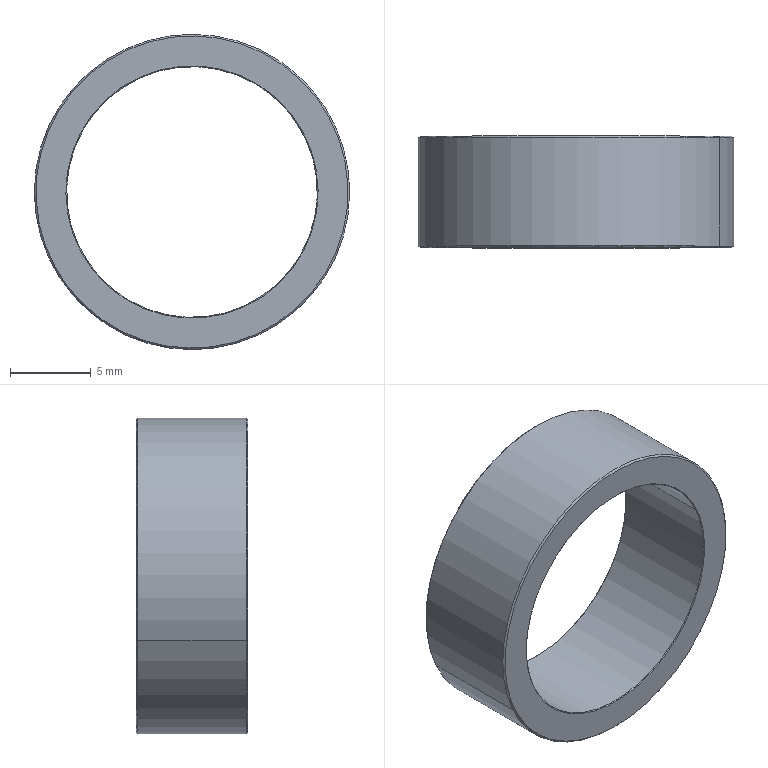Part | SolidWorks | features BaseBody 1 | 1 solid | 14 faces | box 19.5 x 6.9 x 19.5 mm | volume 757.962 mm3 | cone 8 | cylinder 4 | plane 2 | commonest cylinder face diameters 15.5 x2 19.5 x2
STEP:
#1=CARTESIAN_POINT('',(-394.588,-106.1,40.281));
#2=VERTEX_POINT('',#1);
#3=CARTESIAN_POINT('',(-384.335,-106.1,36.407));
#4=VERTEX_POINT('',#3);
#5=CARTESIAN_POINT('',(-387.524,-106.1,43.47));
#6=DIRECTION('',(0.,-1.,0.));
#7=DIRECTION('',(0.,0.,1.));
#8=AXIS2_PLACEMENT_3D('',#5,#6,#7);
#9=CIRCLE('',#8,7.75);
#10=EDGE_CURVE('',#2,#4,#9,.T.);
#11=ORIENTED_EDGE('',*,*,#10,.T.);
#12=CARTESIAN_POINT('',(-384.315,-106.05,36.361));
#13=VERTEX_POINT('',#12);
#14=CARTESIAN_POINT('',(-384.366,-106.175,36.475));
#15=DIRECTION('',(0.291,0.7071,-0.6445));
#16=VECTOR('',#15,1000.);
#17=LINE('',#14,#16);
#18=EDGE_CURVE('',#4,#13,#17,.T.);
#19=ORIENTED_EDGE('',*,*,#18,.T.);
#20=CARTESIAN_POINT('',(-390.734,-106.05,50.579));
#21=VERTEX_POINT('',#20);
#22=CARTESIAN_POINT('',(-387.524,-106.05,43.47));
#23=DIRECTION('',(0.,-1.,0.));
#24=DIRECTION('',(0.,0.,-1.));
#25=AXIS2_PLACEMENT_3D('',#22,#23,#24);
#26=CIRCLE('',#25,7.8);
#27=EDGE_CURVE('',#21,#13,#26,.T.);
#28=ORIENTED_EDGE('',*,*,#27,.F.);
#29=CARTESIAN_POINT('',(-390.714,-106.1,50.533));
#30=VERTEX_POINT('',#29);
#31=CARTESIAN_POINT('',(-390.683,-106.175,50.465));
#32=DIRECTION('',(-0.291,0.7071,0.6445));
#33=VECTOR('',#32,1000.);
#34=LINE('',#31,#33);
#35=EDGE_CURVE('',#30,#21,#34,.T.);
#36=ORIENTED_EDGE('',*,*,#35,.F.);
#37=CARTESIAN_POINT('',(-387.524,-106.1,43.47));
#38=DIRECTION('',(0.,-1.,0.));
#39=DIRECTION('',(0.,0.,1.));
#40=AXIS2_PLACEMENT_3D('',#37,#38,#39);
#41=CIRCLE('',#40,7.75);
#42=EDGE_CURVE('',#30,#2,#41,.T.);
#43=ORIENTED_EDGE('',*,*,#42,.T.);
#44=EDGE_LOOP('',(#11,#19,#28,#36,#43));
#45=FACE_OUTER_BOUND('',#44,.T.);
#46=CARTESIAN_POINT('',(-387.524,-106.175,43.47));
#47=DIRECTION('',(0.,1.,0.));
#48=DIRECTION('',(-0.4115,0.,0.9114));
#49=AXIS2_PLACEMENT_3D('',#46,#47,#48);
#50=CONICAL_SURFACE('',#49,7.675,0.7854);
#51=ADVANCED_FACE('',(#45),#50,.F.);
#52=CARTESIAN_POINT('',(-380.461,-112.9,46.659));
#53=VERTEX_POINT('',#52);
#54=CARTESIAN_POINT('',(-384.335,-112.9,36.407));
#55=VERTEX_POINT('',#54);
#56=CARTESIAN_POINT('',(-387.524,-112.9,43.47));
#57=DIRECTION('',(0.,1.,0.));
#58=DIRECTION('',(0.,0.,-1.));
#59=AXIS2_PLACEMENT_3D('',#56,#57,#58);
#60=CIRCLE('',#59,7.75);
#61=EDGE_CURVE('',#53,#55,#60,.T.);
#62=ORIENTED_EDGE('',*,*,#61,.T.);
#63=CARTESIAN_POINT('',(-384.315,-112.95,36.361));
#64=VERTEX_POINT('',#63);
#65=CARTESIAN_POINT('',(-384.366,-112.825,36.475));
#66=DIRECTION('',(0.291,-0.7071,-0.6445));
#67=VECTOR('',#66,1000.);
#68=LINE('',#65,#67);
#69=EDGE_CURVE('',#55,#64,#68,.T.);
#70=ORIENTED_EDGE('',*,*,#69,.T.);
#71=CARTESIAN_POINT('',(-390.734,-112.95,50.579));
#72=VERTEX_POINT('',#71);
#73=CARTESIAN_POINT('',(-387.524,-112.95,43.47));
#74=DIRECTION('',(0.,1.,0.));
#75=DIRECTION('',(0.,0.,-1.));
#76=AXIS2_PLACEMENT_3D('',#73,#74,#75);
#77=CIRCLE('',#76,7.8);
#78=EDGE_CURVE('',#72,#64,#77,.T.);
#79=ORIENTED_EDGE('',*,*,#78,.F.);
#80=CARTESIAN_POINT('',(-390.714,-112.9,50.533));
#81=VERTEX_POINT('',#80);
#82=CARTESIAN_POINT('',(-390.683,-112.825,50.465));
#83=DIRECTION('',(-0.291,-0.7071,0.6445));
#84=VECTOR('',#83,1000.);
#85=LINE('',#82,#84);
#86=EDGE_CURVE('',#81,#72,#85,.T.);
#87=ORIENTED_EDGE('',*,*,#86,.F.);
#88=CARTESIAN_POINT('',(-387.524,-112.9,43.47));
#89=DIRECTION('',(0.,1.,0.));
#90=DIRECTION('',(0.,0.,-1.));
#91=AXIS2_PLACEMENT_3D('',#88,#89,#90);
#92=CIRCLE('',#91,7.75);
#93=EDGE_CURVE('',#81,#53,#92,.T.);
#94=ORIENTED_EDGE('',*,*,#93,.T.);
#95=EDGE_LOOP('',(#62,#70,#79,#87,#94));
#96=FACE_OUTER_BOUND('',#95,.T.);
#97=CARTESIAN_POINT('',(-387.524,-112.825,43.47));
#98=DIRECTION('',(0.,-1.,0.));
#99=DIRECTION('',(-0.4115,0.,0.9114));
#100=AXIS2_PLACEMENT_3D('',#97,#98,#99);
#101=CONICAL_SURFACE('',#100,7.675,0.7854);
#102=ADVANCED_FACE('',(#96),#101,.F.);
#103=CARTESIAN_POINT('',(-383.553,-112.95,34.675));
#104=VERTEX_POINT('',#103);
#105=CARTESIAN_POINT('',(-391.496,-112.95,52.265));
#106=VERTEX_POINT('',#105);
#107=CARTESIAN_POINT('',(-387.524,-112.95,43.47));
#108=DIRECTION('',(0.,-1.,0.));
#109=DIRECTION('',(0.,0.,-1.));
#110=AXIS2_PLACEMENT_3D('',#107,#108,#109);
#111=CIRCLE('',#110,9.65);
#112=EDGE_CURVE('',#104,#106,#111,.T.);
#113=ORIENTED_EDGE('',*,*,#112,.F.);
#114=CARTESIAN_POINT('',(-383.512,-112.85,34.584));
#115=VERTEX_POINT('',#114);
#116=CARTESIAN_POINT('',(-383.502,-112.825,34.561));
#117=DIRECTION('',(0.291,0.7071,-0.6445));
#118=VECTOR('',#117,1000.);
#119=LINE('',#116,#118);
#120=EDGE_CURVE('',#104,#115,#119,.T.);
#121=ORIENTED_EDGE('',*,*,#120,.T.);
#122=CARTESIAN_POINT('',(-378.638,-112.85,47.482));
#123=VERTEX_POINT('',#122);
#124=CARTESIAN_POINT('',(-387.524,-112.85,43.47));
#125=DIRECTION('',(0.,-1.,0.));
#126=DIRECTION('',(0.,0.,1.));
#127=AXIS2_PLACEMENT_3D('',#124,#125,#126);
#128=CIRCLE('',#127,9.75);
#129=EDGE_CURVE('',#115,#123,#128,.T.);
#130=ORIENTED_EDGE('',*,*,#129,.T.);
#131=CARTESIAN_POINT('',(-391.537,-112.85,52.356));
#132=VERTEX_POINT('',#131);
#133=CARTESIAN_POINT('',(-387.524,-112.85,43.47));
#134=DIRECTION('',(0.,-1.,0.));
#135=DIRECTION('',(0.,0.,1.));
#136=AXIS2_PLACEMENT_3D('',#133,#134,#135);
#137=CIRCLE('',#136,9.75);
#138=EDGE_CURVE('',#123,#132,#137,.T.);
#139=ORIENTED_EDGE('',*,*,#138,.T.);
#140=CARTESIAN_POINT('',(-391.547,-112.825,52.379));
#141=DIRECTION('',(-0.291,0.7071,0.6445));
#142=VECTOR('',#141,1000.);
#143=LINE('',#140,#142);
#144=EDGE_CURVE('',#106,#132,#143,.T.);
#145=ORIENTED_EDGE('',*,*,#144,.F.);
#146=EDGE_LOOP('',(#113,#121,#130,#139,#145));
#147=FACE_OUTER_BOUND('',#146,.T.);
#148=CARTESIAN_POINT('',(-387.524,-112.825,43.47));
#149=DIRECTION('',(0.,1.,0.));
#150=DIRECTION('',(-0.4115,0.,0.9114));
#151=AXIS2_PLACEMENT_3D('',#148,#149,#150);
#152=CONICAL_SURFACE('',#151,9.775,0.7854);
#153=ADVANCED_FACE('',(#147),#152,.T.);
#154=CARTESIAN_POINT('',(-383.553,-106.05,34.675));
#155=VERTEX_POINT('',#154);
#156=CARTESIAN_POINT('',(-391.496,-106.05,52.265));
#157=VERTEX_POINT('',#156);
#158=CARTESIAN_POINT('',(-387.524,-106.05,43.47));
#159=DIRECTION('',(0.,1.,0.));
#160=DIRECTION('',(0.,0.,-1.));
#161=AXIS2_PLACEMENT_3D('',#158,#159,#160);
#162=CIRCLE('',#161,9.65);
#163=EDGE_CURVE('',#155,#157,#162,.T.);
#164=ORIENTED_EDGE('',*,*,#163,.F.);
#165=CARTESIAN_POINT('',(-383.512,-106.15,34.584));
#166=VERTEX_POINT('',#165);
#167=CARTESIAN_POINT('',(-383.502,-106.175,34.561));
#168=DIRECTION('',(0.291,-0.7071,-0.6445));
#169=VECTOR('',#168,1000.);
#170=LINE('',#167,#169);
#171=EDGE_CURVE('',#155,#166,#170,.T.);
#172=ORIENTED_EDGE('',*,*,#171,.T.);
#173=CARTESIAN_POINT('',(-396.411,-106.15,39.458));
#174=VERTEX_POINT('',#173);
#175=CARTESIAN_POINT('',(-387.524,-106.15,43.47));
#176=DIRECTION('',(0.,1.,0.));
#177=DIRECTION('',(0.,0.,-1.));
#178=AXIS2_PLACEMENT_3D('',#175,#176,#177);
#179=CIRCLE('',#178,9.75);
#180=EDGE_CURVE('',#166,#174,#179,.T.);
#181=ORIENTED_EDGE('',*,*,#180,.T.);
#182=CARTESIAN_POINT('',(-391.537,-106.15,52.356));
#183=VERTEX_POINT('',#182);
#184=CARTESIAN_POINT('',(-387.524,-106.15,43.47));
#185=DIRECTION('',(0.,1.,0.));
#186=DIRECTION('',(0.,0.,-1.));
#187=AXIS2_PLACEMENT_3D('',#184,#185,#186);
#188=CIRCLE('',#187,9.75);
#189=EDGE_CURVE('',#174,#183,#188,.T.);
#190=ORIENTED_EDGE('',*,*,#189,.T.);
#191=CARTESIAN_POINT('',(-391.547,-106.175,52.379));
#192=DIRECTION('',(-0.291,-0.7071,0.6445));
#193=VECTOR('',#192,1000.);
#194=LINE('',#191,#193);
#195=EDGE_CURVE('',#157,#183,#194,.T.);
#196=ORIENTED_EDGE('',*,*,#195,.F.);
#197=EDGE_LOOP('',(#164,#172,#181,#190,#196));
#198=FACE_OUTER_BOUND('',#197,.T.);
#199=CARTESIAN_POINT('',(-387.524,-106.175,43.47));
#200=DIRECTION('',(0.,-1.,0.));
#201=DIRECTION('',(-0.4115,0.,0.9114));
#202=AXIS2_PLACEMENT_3D('',#199,#200,#201);
#203=CONICAL_SURFACE('',#202,9.775,0.7854);
#204=ADVANCED_FACE('',(#198),#203,.T.);
#205=CARTESIAN_POINT('',(-378.638,-106.15,47.482));
#206=VERTEX_POINT('',#205);
#207=CARTESIAN_POINT('',(-387.524,-106.15,43.47));
#208=DIRECTION('',(0.,1.,0.));
#209=DIRECTION('',(0.,0.,-1.));
#210=AXIS2_PLACEMENT_3D('',#207,#208,#209);
#211=CIRCLE('',#210,9.75);
#212=EDGE_CURVE('',#206,#166,#211,.T.);
#213=ORIENTED_EDGE('',*,*,#212,.F.);
#214=CARTESIAN_POINT('',(-378.638,-106.,47.482));
#215=DIRECTION('',(0.,-1.,0.));
#216=VECTOR('',#215,1000.);
#217=LINE('',#214,#216);
#218=EDGE_CURVE('',#206,#123,#217,.T.);
#219=ORIENTED_EDGE('',*,*,#218,.T.);
#220=ORIENTED_EDGE('',*,*,#129,.F.);
#221=CARTESIAN_POINT('',(-396.411,-112.85,39.458));
#222=VERTEX_POINT('',#221);
#223=CARTESIAN_POINT('',(-387.524,-112.85,43.47));
#224=DIRECTION('',(0.,-1.,0.));
#225=DIRECTION('',(0.,0.,1.));
#226=AXIS2_PLACEMENT_3D('',#223,#224,#225);
#227=CIRCLE('',#226,9.75);
#228=EDGE_CURVE('',#222,#115,#227,.T.);
#229=ORIENTED_EDGE('',*,*,#228,.F.);
#230=CARTESIAN_POINT('',(-396.411,-106.,39.458));
#231=DIRECTION('',(0.,-1.,0.));
#232=VECTOR('',#231,1000.);
#233=LINE('',#230,#232);
#234=EDGE_CURVE('',#174,#222,#233,.T.);
#235=ORIENTED_EDGE('',*,*,#234,.F.);
#236=ORIENTED_EDGE('',*,*,#180,.F.);
#237=EDGE_LOOP('',(#213,#219,#220,#229,#235,#236));
#238=FACE_OUTER_BOUND('',#237,.T.);
#239=CARTESIAN_POINT('',(-387.524,-106.,43.47));
#240=DIRECTION('',(0.,-1.,0.));
#241=DIRECTION('',(-0.9114,0.,-0.4115));
#242=AXIS2_PLACEMENT_3D('',#239,#240,#241);
#243=CYLINDRICAL_SURFACE('',#242,9.75);
#244=ADVANCED_FACE('',(#238),#243,.T.);
#245=CARTESIAN_POINT('',(-380.461,-106.1,46.659));
#246=VERTEX_POINT('',#245);
#247=CARTESIAN_POINT('',(-387.524,-106.1,43.47));
#248=DIRECTION('',(0.,-1.,0.));
#249=DIRECTION('',(0.,0.,1.));
#250=AXIS2_PLACEMENT_3D('',#247,#248,#249);
#251=CIRCLE('',#250,7.75);
#252=EDGE_CURVE('',#246,#30,#251,.T.);
#253=ORIENTED_EDGE('',*,*,#252,.F.);
#254=CARTESIAN_POINT('',(-380.461,-106.,46.659));
#255=DIRECTION('',(0.,-1.,0.));
#256=VECTOR('',#255,1000.);
#257=LINE('',#254,#256);
#258=EDGE_CURVE('',#246,#53,#257,.T.);
#259=ORIENTED_EDGE('',*,*,#258,.T.);
#260=ORIENTED_EDGE('',*,*,#93,.F.);
#261=CARTESIAN_POINT('',(-394.588,-112.9,40.281));
#262=VERTEX_POINT('',#261);
#263=CARTESIAN_POINT('',(-387.524,-112.9,43.47));
#264=DIRECTION('',(0.,1.,0.));
#265=DIRECTION('',(0.,0.,-1.));
#266=AXIS2_PLACEMENT_3D('',#263,#264,#265);
#267=CIRCLE('',#266,7.75);
#268=EDGE_CURVE('',#262,#81,#267,.T.);
#269=ORIENTED_EDGE('',*,*,#268,.F.);
#270=CARTESIAN_POINT('',(-394.588,-106.,40.281));
#271=DIRECTION('',(0.,-1.,0.));
#272=VECTOR('',#271,1000.);
#273=LINE('',#270,#272);
#274=EDGE_CURVE('',#2,#262,#273,.T.);
#275=ORIENTED_EDGE('',*,*,#274,.F.);
#276=ORIENTED_EDGE('',*,*,#42,.F.);
#277=EDGE_LOOP('',(#253,#259,#260,#269,#275,#276));
#278=FACE_OUTER_BOUND('',#277,.T.);
#279=CARTESIAN_POINT('',(-387.524,-106.,43.47));
#280=DIRECTION('',(0.,-1.,0.));
#281=DIRECTION('',(-0.9114,0.,-0.4115));
#282=AXIS2_PLACEMENT_3D('',#279,#280,#281);
#283=CYLINDRICAL_SURFACE('',#282,7.75);
#284=ADVANCED_FACE('',(#278),#283,.F.);
#285=ORIENTED_EDGE('',*,*,#27,.T.);
#286=CARTESIAN_POINT('',(-387.524,-106.05,43.47));
#287=DIRECTION('',(0.,-1.,0.));
#288=DIRECTION('',(0.,0.,-1.));
#289=AXIS2_PLACEMENT_3D('',#286,#287,#288);
#290=CIRCLE('',#289,7.8);
#291=EDGE_CURVE('',#13,#21,#290,.T.);
#292=ORIENTED_EDGE('',*,*,#291,.T.);
#293=EDGE_LOOP('',(#285,#292));
#294=FACE_BOUND('',#293,.T.);
#295=CARTESIAN_POINT('',(-387.524,-106.05,43.47));
#296=DIRECTION('',(0.,1.,0.));
#297=DIRECTION('',(0.,0.,-1.));
#298=AXIS2_PLACEMENT_3D('',#295,#296,#297);
#299=CIRCLE('',#298,9.65);
#300=EDGE_CURVE('',#157,#155,#299,.T.);
#301=ORIENTED_EDGE('',*,*,#300,.T.);
#302=ORIENTED_EDGE('',*,*,#163,.T.);
#303=EDGE_LOOP('',(#301,#302));
#304=FACE_OUTER_BOUND('',#303,.T.);
#305=CARTESIAN_POINT('',(-21.78,-106.05,172.659));
#306=DIRECTION('',(0.,-1.,0.));
#307=DIRECTION('',(0.,0.,-1.));
#308=AXIS2_PLACEMENT_3D('',#305,#306,#307);
#309=PLANE('',#308);
#310=ADVANCED_FACE('',(#294,#304),#309,.F.);
#311=ORIENTED_EDGE('',*,*,#78,.T.);
#312=CARTESIAN_POINT('',(-387.524,-112.95,43.47));
#313=DIRECTION('',(0.,1.,0.));
#314=DIRECTION('',(0.,0.,-1.));
#315=AXIS2_PLACEMENT_3D('',#312,#313,#314);
#316=CIRCLE('',#315,7.8);
#317=EDGE_CURVE('',#64,#72,#316,.T.);
#318=ORIENTED_EDGE('',*,*,#317,.T.);
#319=EDGE_LOOP('',(#311,#318));
#320=FACE_BOUND('',#319,.T.);
#321=CARTESIAN_POINT('',(-387.524,-112.95,43.47));
#322=DIRECTION('',(0.,-1.,0.));
#323=DIRECTION('',(0.,0.,-1.));
#324=AXIS2_PLACEMENT_3D('',#321,#322,#323);
#325=CIRCLE('',#324,9.65);
#326=EDGE_CURVE('',#106,#104,#325,.T.);
#327=ORIENTED_EDGE('',*,*,#326,.T.);
#328=ORIENTED_EDGE('',*,*,#112,.T.);
#329=EDGE_LOOP('',(#327,#328));
#330=FACE_OUTER_BOUND('',#329,.T.);
#331=CARTESIAN_POINT('',(-21.78,-112.95,172.659));
#332=DIRECTION('',(0.,-1.,0.));
#333=DIRECTION('',(0.,0.,-1.));
#334=AXIS2_PLACEMENT_3D('',#331,#332,#333);
#335=PLANE('',#334);
#336=ADVANCED_FACE('',(#320,#330),#335,.T.);
#337=ORIENTED_EDGE('',*,*,#258,.F.);
#338=CARTESIAN_POINT('',(-387.524,-106.1,43.47));
#339=DIRECTION('',(0.,-1.,0.));
#340=DIRECTION('',(0.,0.,1.));
#341=AXIS2_PLACEMENT_3D('',#338,#339,#340);
#342=CIRCLE('',#341,7.75);
#343=EDGE_CURVE('',#4,#246,#342,.T.);
#344=ORIENTED_EDGE('',*,*,#343,.F.);
#345=ORIENTED_EDGE('',*,*,#10,.F.);
#346=ORIENTED_EDGE('',*,*,#274,.T.);
#347=CARTESIAN_POINT('',(-387.524,-112.9,43.47));
#348=DIRECTION('',(0.,1.,0.));
#349=DIRECTION('',(0.,0.,-1.));
#350=AXIS2_PLACEMENT_3D('',#347,#348,#349);
#351=CIRCLE('',#350,7.75);
#352=EDGE_CURVE('',#55,#262,#351,.T.);
#353=ORIENTED_EDGE('',*,*,#352,.F.);
#354=ORIENTED_EDGE('',*,*,#61,.F.);
#355=EDGE_LOOP('',(#337,#344,#345,#346,#353,#354));
#356=FACE_OUTER_BOUND('',#355,.T.);
#357=CARTESIAN_POINT('',(-387.524,-106.,43.47));
#358=DIRECTION('',(0.,-1.,0.));
#359=DIRECTION('',(-0.9114,0.,-0.4115));
#360=AXIS2_PLACEMENT_3D('',#357,#358,#359);
#361=CYLINDRICAL_SURFACE('',#360,7.75);
#362=ADVANCED_FACE('',(#356),#361,.F.);
#363=ORIENTED_EDGE('',*,*,#218,.F.);
#364=CARTESIAN_POINT('',(-387.524,-106.15,43.47));
#365=DIRECTION('',(0.,1.,0.));
#366=DIRECTION('',(0.,0.,-1.));
#367=AXIS2_PLACEMENT_3D('',#364,#365,#366);
#368=CIRCLE('',#367,9.75);
#369=EDGE_CURVE('',#183,#206,#368,.T.);
#370=ORIENTED_EDGE('',*,*,#369,.F.);
#371=ORIENTED_EDGE('',*,*,#189,.F.);
#372=ORIENTED_EDGE('',*,*,#234,.T.);
#373=CARTESIAN_POINT('',(-387.524,-112.85,43.47));
#374=DIRECTION('',(0.,-1.,0.));
#375=DIRECTION('',(0.,0.,1.));
#376=AXIS2_PLACEMENT_3D('',#373,#374,#375);
#377=CIRCLE('',#376,9.75);
#378=EDGE_CURVE('',#132,#222,#377,.T.);
#379=ORIENTED_EDGE('',*,*,#378,.F.);
#380=ORIENTED_EDGE('',*,*,#138,.F.);
#381=EDGE_LOOP('',(#363,#370,#371,#372,#379,#380));
#382=FACE_OUTER_BOUND('',#381,.T.);
#383=CARTESIAN_POINT('',(-387.524,-106.,43.47));
#384=DIRECTION('',(0.,-1.,0.));
#385=DIRECTION('',(-0.9114,0.,-0.4115));
#386=AXIS2_PLACEMENT_3D('',#383,#384,#385);
#387=CYLINDRICAL_SURFACE('',#386,9.75);
#388=ADVANCED_FACE('',(#382),#387,.T.);
#389=ORIENTED_EDGE('',*,*,#171,.F.);
#390=ORIENTED_EDGE('',*,*,#300,.F.);
#391=ORIENTED_EDGE('',*,*,#195,.T.);
#392=ORIENTED_EDGE('',*,*,#369,.T.);
#393=ORIENTED_EDGE('',*,*,#212,.T.);
#394=EDGE_LOOP('',(#389,#390,#391,#392,#393));
#395=FACE_OUTER_BOUND('',#394,.T.);
#396=CARTESIAN_POINT('',(-387.524,-106.175,43.47));
#397=DIRECTION('',(0.,-1.,0.));
#398=DIRECTION('',(-0.4115,0.,0.9114));
#399=AXIS2_PLACEMENT_3D('',#396,#397,#398);
#400=CONICAL_SURFACE('',#399,9.775,0.7854);
#401=ADVANCED_FACE('',(#395),#400,.T.);
#402=ORIENTED_EDGE('',*,*,#120,.F.);
#403=ORIENTED_EDGE('',*,*,#326,.F.);
#404=ORIENTED_EDGE('',*,*,#144,.T.);
#405=ORIENTED_EDGE('',*,*,#378,.T.);
#406=ORIENTED_EDGE('',*,*,#228,.T.);
#407=EDGE_LOOP('',(#402,#403,#404,#405,#406));
#408=FACE_OUTER_BOUND('',#407,.T.);
#409=CARTESIAN_POINT('',(-387.524,-112.825,43.47));
#410=DIRECTION('',(0.,1.,0.));
#411=DIRECTION('',(-0.4115,0.,0.9114));
#412=AXIS2_PLACEMENT_3D('',#409,#410,#411);
#413=CONICAL_SURFACE('',#412,9.775,0.7854);
#414=ADVANCED_FACE('',(#408),#413,.T.);
#415=ORIENTED_EDGE('',*,*,#69,.F.);
#416=ORIENTED_EDGE('',*,*,#352,.T.);
#417=ORIENTED_EDGE('',*,*,#268,.T.);
#418=ORIENTED_EDGE('',*,*,#86,.T.);
#419=ORIENTED_EDGE('',*,*,#317,.F.);
#420=EDGE_LOOP('',(#415,#416,#417,#418,#419));
#421=FACE_OUTER_BOUND('',#420,.T.);
#422=CARTESIAN_POINT('',(-387.524,-112.825,43.47));
#423=DIRECTION('',(0.,-1.,0.));
#424=DIRECTION('',(-0.4115,0.,0.9114));
#425=AXIS2_PLACEMENT_3D('',#422,#423,#424);
#426=CONICAL_SURFACE('',#425,7.675,0.7854);
#427=ADVANCED_FACE('',(#421),#426,.F.);
#428=ORIENTED_EDGE('',*,*,#18,.F.);
#429=ORIENTED_EDGE('',*,*,#343,.T.);
#430=ORIENTED_EDGE('',*,*,#252,.T.);
#431=ORIENTED_EDGE('',*,*,#35,.T.);
#432=ORIENTED_EDGE('',*,*,#291,.F.);
#433=EDGE_LOOP('',(#428,#429,#430,#431,#432));
#434=FACE_OUTER_BOUND('',#433,.T.);
#435=CARTESIAN_POINT('',(-387.524,-106.175,43.47));
#436=DIRECTION('',(0.,1.,0.));
#437=DIRECTION('',(-0.4115,0.,0.9114));
#438=AXIS2_PLACEMENT_3D('',#435,#436,#437);
#439=CONICAL_SURFACE('',#438,7.675,0.7854);
#440=ADVANCED_FACE('',(#434),#439,.F.);
#441=CLOSED_SHELL('',(#51,#102,#153,#204,#244,#284,#310,#336,#362,#388,#401,#414,#427,#440));
#442=MANIFOLD_SOLID_BREP('',#441);
#443=CARTESIAN_POINT('',(0.,0.,0.));
#444=DIRECTION('',(0.,0.,1.));
#445=DIRECTION('',(1.,0.,0.));
#446=AXIS2_PLACEMENT_3D('',#443,#444,#445);
#447=(LENGTH_UNIT()NAMED_UNIT(*)SI_UNIT(.MILLI.,.METRE.));
#448=UNCERTAINTY_MEASURE_WITH_UNIT(LENGTH_MEASURE(0.00001),#447,'','');
#449=(NAMED_UNIT(*)PLANE_ANGLE_UNIT()SI_UNIT($,.RADIAN.));
#450=(NAMED_UNIT(*)SI_UNIT($,.STERADIAN.)SOLID_ANGLE_UNIT());
#451=(GEOMETRIC_REPRESENTATION_CONTEXT(3)GLOBAL_UNCERTAINTY_ASSIGNED_CONTEXT((#448))GLOBAL_UNIT_ASSIGNED_CONTEXT((#447,#449,#450))REPRESENTATION_CONTEXT('',''));
#452=ADVANCED_BREP_SHAPE_REPRESENTATION('',(#442,#446),#451);